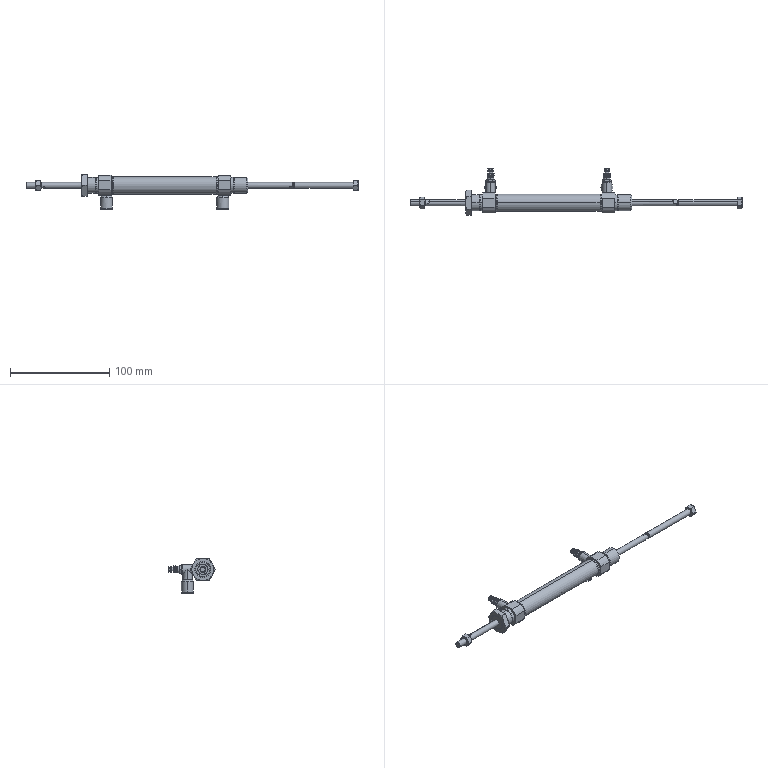Part | SolidWorks | 7 solids | 1090 faces | box 334 x 47.242 x 35.2 mm | volume 41085 mm3 | cylinder 630 | spline 250 | plane 124 | cone 86 | commonest cylinder face diameters 0.494 x150 0.716 x140 4.724 x56 5.2 x56 6.564 x56 7.04 x56